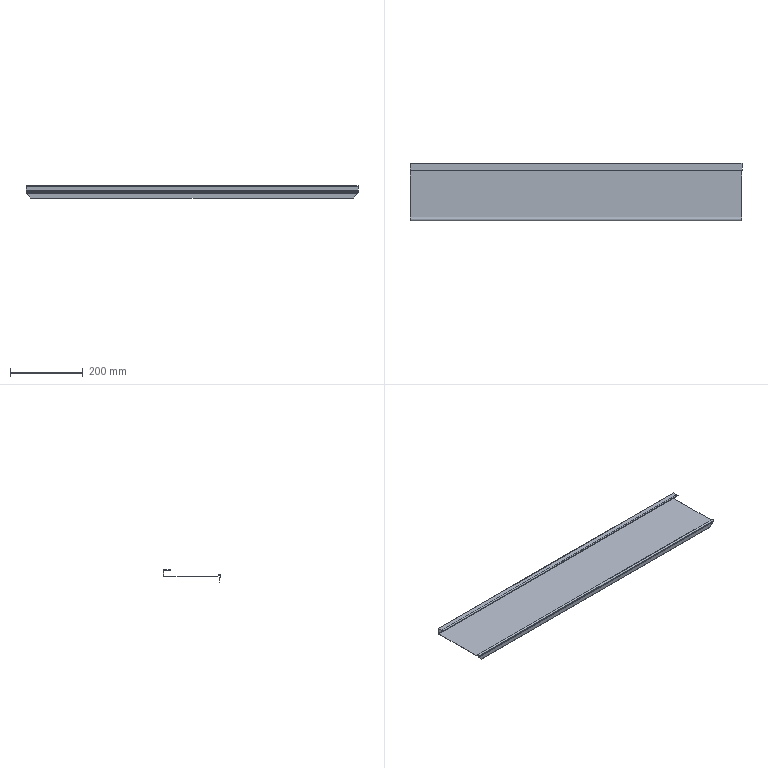Part | SolidWorks | features SM3dBend 4, EdgeFlange 2, FlatPattern 1, Hem 1, SMBaseFlange 1, SheetMetal 1 | 1 solid | 64 faces | box 915 x 157.414 x 33.2 mm | volume 160931 mm3 | plane 48 | cylinder 14 | spline 2 | commonest cylinder face diameters 1 x3 2.6 x3 0.1 x1 1.2 x1 1.7 x1 2.8 x1